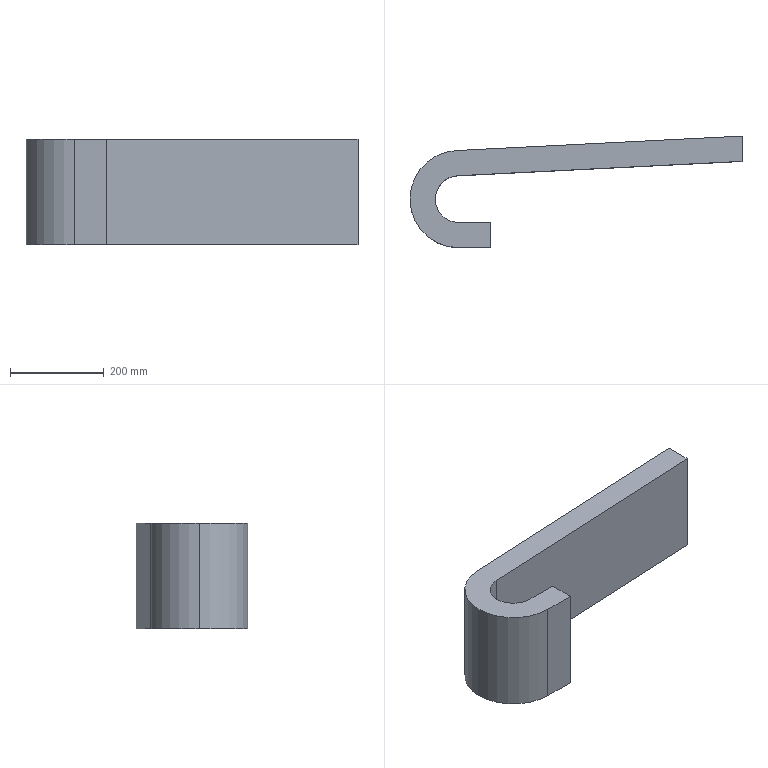Part | STEP file | TKR26H40W200R75+35L-FU-MU-Part-1 | 1 solid | 24 faces | box 710 x 238.7 x 226 mm | volume 3855822 mm3 | plane 16 | cylinder 8 | commonest cylinder face diameters 100 x2 114 x2 194 x2 208 x2